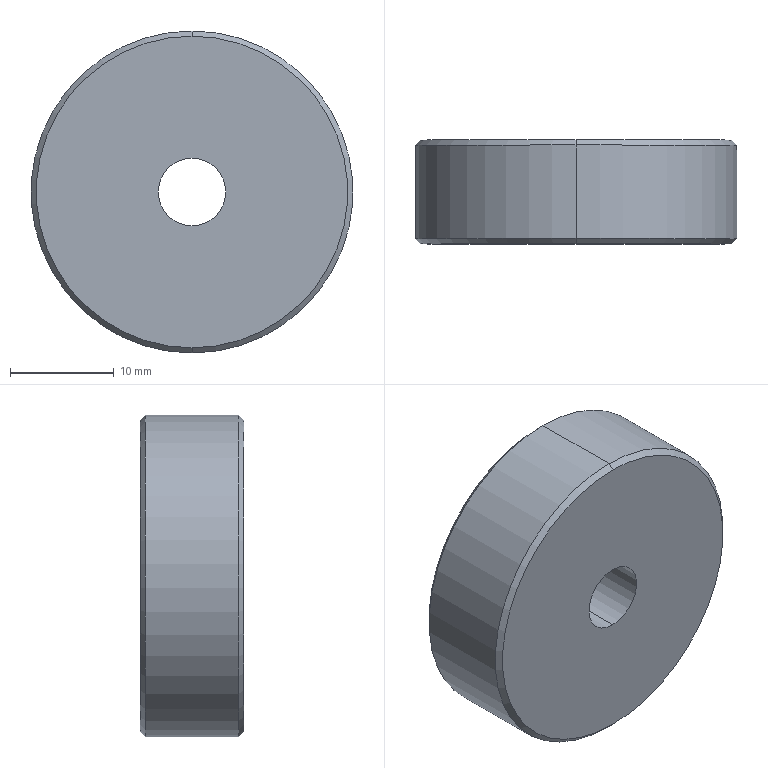Part | STEP file | OP10-124_seal pad | 1 solid | 13 faces | box 31 x 10 x 31 mm | volume 7003 mm3 | cylinder 6 | cone 4 | plane 3 | commonest cylinder face diameters 6.5 x2 9.5 x2 31 x2
STEP:
#1=CARTESIAN_POINT('',(0.,0.,0.));
#2=DIRECTION('',(0.,0.,1.));
#3=DIRECTION('',(1.,0.,0.));
#4=AXIS2_PLACEMENT_3D('',#1,#2,#3);
#5=CARTESIAN_POINT('',(0.,10.,15.));
#6=VERTEX_POINT('',#5);
#7=CARTESIAN_POINT('',(0.,10.,-15.));
#8=VERTEX_POINT('',#7);
#9=CARTESIAN_POINT('',(0.,10.,0.));
#10=DIRECTION('',(0.,1.,0.));
#11=DIRECTION('',(0.,0.,1.));
#12=AXIS2_PLACEMENT_3D('',#9,#10,#11);
#13=CIRCLE('',#12,15.);
#14=CARTESIAN_POINT('',(0.,10.,0.));
#15=DIRECTION('',(0.,-1.,0.));
#16=DIRECTION('',(0.,0.,-1.));
#17=AXIS2_PLACEMENT_3D('',#14,#15,#16);
#18=CONICAL_SURFACE('',#17,15.,0.7854);
#19=CARTESIAN_POINT('',(3.142,0.));
#20=DIRECTION('',(-1.,0.));
#21=VECTOR('',#20,1.);
#22=LINE('',#19,#21);
#23=(GEOMETRIC_REPRESENTATION_CONTEXT(2)PARAMETRIC_REPRESENTATION_CONTEXT()REPRESENTATION_CONTEXT('',''));
#24=DEFINITIONAL_REPRESENTATION('',(#22),#23);
#25=PCURVE('',#18,#24);
#26=CARTESIAN_POINT('',(0.,10.,0.));
#27=DIRECTION('',(0.,1.,0.));
#28=DIRECTION('',(0.,0.,1.));
#29=AXIS2_PLACEMENT_3D('',#26,#27,#28);
#30=PLANE('',#29);
#31=CARTESIAN_POINT('',(0.,0.));
#32=DIRECTION('',(1.,0.));
#33=AXIS2_PLACEMENT_2D('',#31,#32);
#34=CIRCLE('',#33,15.);
#35=(GEOMETRIC_REPRESENTATION_CONTEXT(2)PARAMETRIC_REPRESENTATION_CONTEXT()REPRESENTATION_CONTEXT('',''));
#36=DEFINITIONAL_REPRESENTATION('',(#34),#35);
#37=PCURVE('',#30,#36);
#38=SURFACE_CURVE('',#13,(#25,#37),.PCURVE_S1.);
#39=EDGE_CURVE('',#6,#8,#38,.T.);
#40=ORIENTED_EDGE('',*,*,#39,.F.);
#41=CARTESIAN_POINT('',(0.,9.5,15.5));
#42=VERTEX_POINT('',#41);
#43=CARTESIAN_POINT('',(0.,10.,15.));
#44=DIRECTION('',(0.,-0.7071,0.7071));
#45=VECTOR('',#44,1.);
#46=LINE('',#43,#45);
#47=CARTESIAN_POINT('',(3.142,0.));
#48=DIRECTION('',(0.,1.));
#49=VECTOR('',#48,1.);
#50=LINE('',#47,#49);
#51=(GEOMETRIC_REPRESENTATION_CONTEXT(2)PARAMETRIC_REPRESENTATION_CONTEXT()REPRESENTATION_CONTEXT('',''));
#52=DEFINITIONAL_REPRESENTATION('',(#50),#51);
#53=PCURVE('',#18,#52);
#54=CARTESIAN_POINT('',(0.,10.,0.));
#55=DIRECTION('',(0.,-1.,0.));
#56=DIRECTION('',(0.,0.,-1.));
#57=AXIS2_PLACEMENT_3D('',#54,#55,#56);
#58=CONICAL_SURFACE('',#57,15.,0.7854);
#59=CARTESIAN_POINT('',(3.142,0.));
#60=DIRECTION('',(0.,1.));
#61=VECTOR('',#60,1.);
#62=LINE('',#59,#61);
#63=(GEOMETRIC_REPRESENTATION_CONTEXT(2)PARAMETRIC_REPRESENTATION_CONTEXT()REPRESENTATION_CONTEXT('',''));
#64=DEFINITIONAL_REPRESENTATION('',(#62),#63);
#65=PCURVE('',#58,#64);
#66=SURFACE_CURVE('',#46,(#53,#65),.PCURVE_S1.);
#67=EDGE_CURVE('',#6,#42,#66,.T.);
#68=ORIENTED_EDGE('',*,*,#67,.T.);
#69=CARTESIAN_POINT('',(0.,9.5,-15.5));
#70=VERTEX_POINT('',#69);
#71=CARTESIAN_POINT('',(0.,9.5,0.));
#72=DIRECTION('',(0.,-1.,0.));
#73=DIRECTION('',(0.,0.,1.));
#74=AXIS2_PLACEMENT_3D('',#71,#72,#73);
#75=CIRCLE('',#74,15.5);
#76=CARTESIAN_POINT('',(-3.142,0.5));
#77=DIRECTION('',(1.,0.));
#78=VECTOR('',#77,1.);
#79=LINE('',#76,#78);
#80=(GEOMETRIC_REPRESENTATION_CONTEXT(2)PARAMETRIC_REPRESENTATION_CONTEXT()REPRESENTATION_CONTEXT('',''));
#81=DEFINITIONAL_REPRESENTATION('',(#79),#80);
#82=PCURVE('',#18,#81);
#83=CARTESIAN_POINT('',(0.,10.,0.));
#84=DIRECTION('',(0.,-1.,0.));
#85=DIRECTION('',(0.,0.,-1.));
#86=AXIS2_PLACEMENT_3D('',#83,#84,#85);
#87=CYLINDRICAL_SURFACE('',#86,15.5);
#88=CARTESIAN_POINT('',(-3.142,0.5));
#89=DIRECTION('',(1.,0.));
#90=VECTOR('',#89,1.);
#91=LINE('',#88,#90);
#92=(GEOMETRIC_REPRESENTATION_CONTEXT(2)PARAMETRIC_REPRESENTATION_CONTEXT()REPRESENTATION_CONTEXT('',''));
#93=DEFINITIONAL_REPRESENTATION('',(#91),#92);
#94=PCURVE('',#87,#93);
#95=SURFACE_CURVE('',#75,(#82,#94),.PCURVE_S1.);
#96=EDGE_CURVE('',#70,#42,#95,.T.);
#97=ORIENTED_EDGE('',*,*,#96,.F.);
#98=CARTESIAN_POINT('',(0.,10.,-15.));
#99=DIRECTION('',(0.,-0.7071,-0.7071));
#100=VECTOR('',#99,1.);
#101=LINE('',#98,#100);
#102=CARTESIAN_POINT('',(0.,0.));
#103=DIRECTION('',(0.,1.));
#104=VECTOR('',#103,1.);
#105=LINE('',#102,#104);
#106=(GEOMETRIC_REPRESENTATION_CONTEXT(2)PARAMETRIC_REPRESENTATION_CONTEXT()REPRESENTATION_CONTEXT('',''));
#107=DEFINITIONAL_REPRESENTATION('',(#105),#106);
#108=PCURVE('',#18,#107);
#109=CARTESIAN_POINT('',(6.283,0.));
#110=DIRECTION('',(0.,1.));
#111=VECTOR('',#110,1.);
#112=LINE('',#109,#111);
#113=(GEOMETRIC_REPRESENTATION_CONTEXT(2)PARAMETRIC_REPRESENTATION_CONTEXT()REPRESENTATION_CONTEXT('',''));
#114=DEFINITIONAL_REPRESENTATION('',(#112),#113);
#115=PCURVE('',#58,#114);
#116=SURFACE_CURVE('',#101,(#108,#115),.PCURVE_S1.);
#117=EDGE_CURVE('',#8,#70,#116,.T.);
#118=ORIENTED_EDGE('',*,*,#117,.F.);
#119=EDGE_LOOP('',(#40,#68,#97,#118));
#120=FACE_BOUND('',#119,.T.);
#121=ADVANCED_FACE('',(#120),#18,.T.);
#122=CARTESIAN_POINT('',(0.,0.,-15.));
#123=VERTEX_POINT('',#122);
#124=CARTESIAN_POINT('',(0.,0.,15.));
#125=VERTEX_POINT('',#124);
#126=CARTESIAN_POINT('',(0.,0.,0.));
#127=DIRECTION('',(0.,-1.,0.));
#128=DIRECTION('',(0.,0.,1.));
#129=AXIS2_PLACEMENT_3D('',#126,#127,#128);
#130=CIRCLE('',#129,15.);
#131=CARTESIAN_POINT('',(0.,0.5,0.));
#132=DIRECTION('',(0.,1.,0.));
#133=DIRECTION('',(0.,0.,1.));
#134=AXIS2_PLACEMENT_3D('',#131,#132,#133);
#135=CONICAL_SURFACE('',#134,15.5,0.7854);
#136=CARTESIAN_POINT('',(6.283,-0.5));
#137=DIRECTION('',(-1.,0.));
#138=VECTOR('',#137,1.);
#139=LINE('',#136,#138);
#140=(GEOMETRIC_REPRESENTATION_CONTEXT(2)PARAMETRIC_REPRESENTATION_CONTEXT()REPRESENTATION_CONTEXT('',''));
#141=DEFINITIONAL_REPRESENTATION('',(#139),#140);
#142=PCURVE('',#135,#141);
#143=CARTESIAN_POINT('',(0.,0.,0.));
#144=DIRECTION('',(0.,1.,0.));
#145=DIRECTION('',(0.,0.,1.));
#146=AXIS2_PLACEMENT_3D('',#143,#144,#145);
#147=PLANE('',#146);
#148=CARTESIAN_POINT('',(15.,0.));
#149=CARTESIAN_POINT('',(15.,-25.981));
#150=CARTESIAN_POINT('',(-7.5,-12.99));
#151=CARTESIAN_POINT('',(-30.,0.));
#152=CARTESIAN_POINT('',(-7.5,12.99));
#153=CARTESIAN_POINT('',(15.,25.981));
#154=CARTESIAN_POINT('',(15.,0.));
#155=(BOUNDED_CURVE()B_SPLINE_CURVE(2,(#148,#149,#150,#151,#152,#153,#154),.UNSPECIFIED.,.T.,.F.)B_SPLINE_CURVE_WITH_KNOTS((1,2,2,2,2,1),(-2.094,0.,2.094,4.189,6.283,8.378),.UNSPECIFIED.)CURVE()GEOMETRIC_REPRESENTATION_ITEM()RATIONAL_B_SPLINE_CURVE((1.,0.5,1.,0.5,1.,0.5,1.))REPRESENTATION_ITEM(''));
#156=(GEOMETRIC_REPRESENTATION_CONTEXT(2)PARAMETRIC_REPRESENTATION_CONTEXT()REPRESENTATION_CONTEXT('',''));
#157=DEFINITIONAL_REPRESENTATION('',(#155),#156);
#158=PCURVE('',#147,#157);
#159=SURFACE_CURVE('',#130,(#142,#158),.PCURVE_S1.);
#160=EDGE_CURVE('',#123,#125,#159,.T.);
#161=ORIENTED_EDGE('',*,*,#160,.F.);
#162=CARTESIAN_POINT('',(0.,0.5,-15.5));
#163=VERTEX_POINT('',#162);
#164=CARTESIAN_POINT('',(0.,0.5,-15.5));
#165=DIRECTION('',(0.,0.7071,-0.7071));
#166=VECTOR('',#165,1.);
#167=LINE('',#164,#166);
#168=CARTESIAN_POINT('',(3.142,0.));
#169=DIRECTION('',(0.,1.));
#170=VECTOR('',#169,1.);
#171=LINE('',#168,#170);
#172=(GEOMETRIC_REPRESENTATION_CONTEXT(2)PARAMETRIC_REPRESENTATION_CONTEXT()REPRESENTATION_CONTEXT('',''));
#173=DEFINITIONAL_REPRESENTATION('',(#171),#172);
#174=PCURVE('',#135,#173);
#175=CARTESIAN_POINT('',(0.,0.5,0.));
#176=DIRECTION('',(0.,1.,0.));
#177=DIRECTION('',(0.,0.,1.));
#178=AXIS2_PLACEMENT_3D('',#175,#176,#177);
#179=CONICAL_SURFACE('',#178,15.5,0.7854);
#180=CARTESIAN_POINT('',(3.142,0.));
#181=DIRECTION('',(0.,1.));
#182=VECTOR('',#181,1.);
#183=LINE('',#180,#182);
#184=(GEOMETRIC_REPRESENTATION_CONTEXT(2)PARAMETRIC_REPRESENTATION_CONTEXT()REPRESENTATION_CONTEXT('',''));
#185=DEFINITIONAL_REPRESENTATION('',(#183),#184);
#186=PCURVE('',#179,#185);
#187=SURFACE_CURVE('',#167,(#174,#186),.PCURVE_S1.);
#188=EDGE_CURVE('',#123,#163,#187,.T.);
#189=ORIENTED_EDGE('',*,*,#188,.T.);
#190=CARTESIAN_POINT('',(0.,0.5,15.5));
#191=VERTEX_POINT('',#190);
#192=CARTESIAN_POINT('',(0.,0.5,0.));
#193=DIRECTION('',(0.,1.,0.));
#194=DIRECTION('',(0.,0.,1.));
#195=AXIS2_PLACEMENT_3D('',#192,#193,#194);
#196=CIRCLE('',#195,15.5);
#197=CARTESIAN_POINT('',(0.,0.));
#198=DIRECTION('',(1.,0.));
#199=VECTOR('',#198,1.);
#200=LINE('',#197,#199);
#201=(GEOMETRIC_REPRESENTATION_CONTEXT(2)PARAMETRIC_REPRESENTATION_CONTEXT()REPRESENTATION_CONTEXT('',''));
#202=DEFINITIONAL_REPRESENTATION('',(#200),#201);
#203=PCURVE('',#135,#202);
#204=CARTESIAN_POINT('',(3.142,9.5));
#205=DIRECTION('',(-1.,0.));
#206=VECTOR('',#205,1.);
#207=LINE('',#204,#206);
#208=(GEOMETRIC_REPRESENTATION_CONTEXT(2)PARAMETRIC_REPRESENTATION_CONTEXT()REPRESENTATION_CONTEXT('',''));
#209=DEFINITIONAL_REPRESENTATION('',(#207),#208);
#210=PCURVE('',#87,#209);
#211=SURFACE_CURVE('',#196,(#203,#210),.PCURVE_S1.);
#212=EDGE_CURVE('',#191,#163,#211,.T.);
#213=ORIENTED_EDGE('',*,*,#212,.F.);
#214=CARTESIAN_POINT('',(0.,0.5,15.5));
#215=DIRECTION('',(0.,0.7071,0.7071));
#216=VECTOR('',#215,1.);
#217=LINE('',#214,#216);
#218=CARTESIAN_POINT('',(0.,0.));
#219=DIRECTION('',(0.,1.));
#220=VECTOR('',#219,1.);
#221=LINE('',#218,#220);
#222=(GEOMETRIC_REPRESENTATION_CONTEXT(2)PARAMETRIC_REPRESENTATION_CONTEXT()REPRESENTATION_CONTEXT('',''));
#223=DEFINITIONAL_REPRESENTATION('',(#221),#222);
#224=PCURVE('',#135,#223);
#225=CARTESIAN_POINT('',(6.283,0.));
#226=DIRECTION('',(0.,1.));
#227=VECTOR('',#226,1.);
#228=LINE('',#225,#227);
#229=(GEOMETRIC_REPRESENTATION_CONTEXT(2)PARAMETRIC_REPRESENTATION_CONTEXT()REPRESENTATION_CONTEXT('',''));
#230=DEFINITIONAL_REPRESENTATION('',(#228),#229);
#231=PCURVE('',#179,#230);
#232=SURFACE_CURVE('',#217,(#224,#231),.PCURVE_S1.);
#233=EDGE_CURVE('',#125,#191,#232,.T.);
#234=ORIENTED_EDGE('',*,*,#233,.F.);
#235=EDGE_LOOP('',(#161,#189,#213,#234));
#236=FACE_BOUND('',#235,.T.);
#237=ADVANCED_FACE('',(#236),#135,.T.);
#238=CARTESIAN_POINT('',(0.,5.,4.75));
#239=VERTEX_POINT('',#238);
#240=CARTESIAN_POINT('',(0.,10.,4.75));
#241=VERTEX_POINT('',#240);
#242=CARTESIAN_POINT('',(0.,5.,4.75));
#243=DIRECTION('',(0.,1.,0.));
#244=VECTOR('',#243,1.);
#245=LINE('',#242,#244);
#246=CARTESIAN_POINT('',(0.,5.,0.));
#247=DIRECTION('',(0.,1.,0.));
#248=DIRECTION('',(0.,0.,1.));
#249=AXIS2_PLACEMENT_3D('',#246,#247,#248);
#250=CYLINDRICAL_SURFACE('',#249,4.75);
#251=CARTESIAN_POINT('',(6.283,0.));
#252=DIRECTION('',(0.,1.));
#253=VECTOR('',#252,1.);
#254=LINE('',#251,#253);
#255=(GEOMETRIC_REPRESENTATION_CONTEXT(2)PARAMETRIC_REPRESENTATION_CONTEXT()REPRESENTATION_CONTEXT('',''));
#256=DEFINITIONAL_REPRESENTATION('',(#254),#255);
#257=PCURVE('',#250,#256);
#258=CARTESIAN_POINT('',(0.,5.,0.));
#259=DIRECTION('',(0.,1.,0.));
#260=DIRECTION('',(0.,0.,1.));
#261=AXIS2_PLACEMENT_3D('',#258,#259,#260);
#262=CYLINDRICAL_SURFACE('',#261,4.75);
#263=CARTESIAN_POINT('',(0.,0.));
#264=DIRECTION('',(0.,1.));
#265=VECTOR('',#264,1.);
#266=LINE('',#263,#265);
#267=(GEOMETRIC_REPRESENTATION_CONTEXT(2)PARAMETRIC_REPRESENTATION_CONTEXT()REPRESENTATION_CONTEXT('',''));
#268=DEFINITIONAL_REPRESENTATION('',(#266),#267);
#269=PCURVE('',#262,#268);
#270=SURFACE_CURVE('',#245,(#257,#269),.PCURVE_S1.);
#271=EDGE_CURVE('',#239,#241,#270,.T.);
#272=ORIENTED_EDGE('',*,*,#271,.T.);
#273=CARTESIAN_POINT('',(0.,10.,-4.75));
#274=VERTEX_POINT('',#273);
#275=CARTESIAN_POINT('',(0.,10.,0.));
#276=DIRECTION('',(0.,1.,0.));
#277=DIRECTION('',(0.,0.,1.));
#278=AXIS2_PLACEMENT_3D('',#275,#276,#277);
#279=CIRCLE('',#278,4.75);
#280=CARTESIAN_POINT('',(0.,5.));
#281=DIRECTION('',(1.,0.));
#282=VECTOR('',#281,1.);
#283=LINE('',#280,#282);
#284=(GEOMETRIC_REPRESENTATION_CONTEXT(2)PARAMETRIC_REPRESENTATION_CONTEXT()REPRESENTATION_CONTEXT('',''));
#285=DEFINITIONAL_REPRESENTATION('',(#283),#284);
#286=PCURVE('',#250,#285);
#287=CARTESIAN_POINT('',(0.,0.));
#288=DIRECTION('',(1.,0.));
#289=AXIS2_PLACEMENT_2D('',#287,#288);
#290=CIRCLE('',#289,4.75);
#291=(GEOMETRIC_REPRESENTATION_CONTEXT(2)PARAMETRIC_REPRESENTATION_CONTEXT()REPRESENTATION_CONTEXT('',''));
#292=DEFINITIONAL_REPRESENTATION('',(#290),#291);
#293=PCURVE('',#30,#292);
#294=SURFACE_CURVE('',#279,(#286,#293),.PCURVE_S1.);
#295=EDGE_CURVE('',#274,#241,#294,.T.);
#296=ORIENTED_EDGE('',*,*,#295,.F.);
#297=CARTESIAN_POINT('',(0.,5.,-4.75));
#298=VERTEX_POINT('',#297);
#299=CARTESIAN_POINT('',(0.,5.,-4.75));
#300=DIRECTION('',(0.,1.,0.));
#301=VECTOR('',#300,1.);
#302=LINE('',#299,#301);
#303=CARTESIAN_POINT('',(3.142,0.));
#304=DIRECTION('',(0.,1.));
#305=VECTOR('',#304,1.);
#306=LINE('',#303,#305);
#307=(GEOMETRIC_REPRESENTATION_CONTEXT(2)PARAMETRIC_REPRESENTATION_CONTEXT()REPRESENTATION_CONTEXT('',''));
#308=DEFINITIONAL_REPRESENTATION('',(#306),#307);
#309=PCURVE('',#250,#308);
#310=CARTESIAN_POINT('',(3.142,0.));
#311=DIRECTION('',(0.,1.));
#312=VECTOR('',#311,1.);
#313=LINE('',#310,#312);
#314=(GEOMETRIC_REPRESENTATION_CONTEXT(2)PARAMETRIC_REPRESENTATION_CONTEXT()REPRESENTATION_CONTEXT('',''));
#315=DEFINITIONAL_REPRESENTATION('',(#313),#314);
#316=PCURVE('',#262,#315);
#317=SURFACE_CURVE('',#302,(#309,#316),.PCURVE_S1.);
#318=EDGE_CURVE('',#298,#274,#317,.T.);
#319=ORIENTED_EDGE('',*,*,#318,.F.);
#320=CARTESIAN_POINT('',(0.,5.,0.));
#321=DIRECTION('',(0.,1.,0.));
#322=DIRECTION('',(0.,0.,1.));
#323=AXIS2_PLACEMENT_3D('',#320,#321,#322);
#324=CIRCLE('',#323,4.75);
#325=CARTESIAN_POINT('',(0.,0.));
#326=DIRECTION('',(1.,0.));
#327=VECTOR('',#326,1.);
#328=LINE('',#325,#327);
#329=(GEOMETRIC_REPRESENTATION_CONTEXT(2)PARAMETRIC_REPRESENTATION_CONTEXT()REPRESENTATION_CONTEXT('',''));
#330=DEFINITIONAL_REPRESENTATION('',(#328),#329);
#331=PCURVE('',#250,#330);
#332=CARTESIAN_POINT('',(0.,5.,0.));
#333=DIRECTION('',(0.,1.,0.));
#334=DIRECTION('',(0.,0.,1.));
#335=AXIS2_PLACEMENT_3D('',#332,#333,#334);
#336=PLANE('',#335);
#337=CARTESIAN_POINT('',(0.,0.));
#338=DIRECTION('',(1.,0.));
#339=AXIS2_PLACEMENT_2D('',#337,#338);
#340=CIRCLE('',#339,4.75);
#341=(GEOMETRIC_REPRESENTATION_CONTEXT(2)PARAMETRIC_REPRESENTATION_CONTEXT()REPRESENTATION_CONTEXT('',''));
#342=DEFINITIONAL_REPRESENTATION('',(#340),#341);
#343=PCURVE('',#336,#342);
#344=SURFACE_CURVE('',#324,(#331,#343),.PCURVE_S1.);
#345=EDGE_CURVE('',#298,#239,#344,.T.);
#346=ORIENTED_EDGE('',*,*,#345,.T.);
#347=EDGE_LOOP('',(#272,#296,#319,#346));
#348=FACE_BOUND('',#347,.F.);
#349=ADVANCED_FACE('',(#348),#250,.F.);
#350=ORIENTED_EDGE('',*,*,#96,.T.);
#351=CARTESIAN_POINT('',(0.,10.,15.5));
#352=DIRECTION('',(0.,-1.,0.));
#353=VECTOR('',#352,1.);
#354=LINE('',#351,#353);
#355=CARTESIAN_POINT('',(3.142,0.));
#356=DIRECTION('',(0.,1.));
#357=VECTOR('',#356,1.);
#358=LINE('',#355,#357);
#359=(GEOMETRIC_REPRESENTATION_CONTEXT(2)PARAMETRIC_REPRESENTATION_CONTEXT()REPRESENTATION_CONTEXT('',''));
#360=DEFINITIONAL_REPRESENTATION('',(#358),#359);
#361=PCURVE('',#87,#360);
#362=CARTESIAN_POINT('',(0.,10.,0.));
#363=DIRECTION('',(0.,-1.,0.));
#364=DIRECTION('',(0.,0.,-1.));
#365=AXIS2_PLACEMENT_3D('',#362,#363,#364);
#366=CYLINDRICAL_SURFACE('',#365,15.5);
#367=CARTESIAN_POINT('',(3.142,0.));
#368=DIRECTION('',(0.,1.));
#369=VECTOR('',#368,1.);
#370=LINE('',#367,#369);
#371=(GEOMETRIC_REPRESENTATION_CONTEXT(2)PARAMETRIC_REPRESENTATION_CONTEXT()REPRESENTATION_CONTEXT('',''));
#372=DEFINITIONAL_REPRESENTATION('',(#370),#371);
#373=PCURVE('',#366,#372);
#374=SURFACE_CURVE('',#354,(#361,#373),.PCURVE_S1.);
#375=EDGE_CURVE('',#42,#191,#374,.T.);
#376=ORIENTED_EDGE('',*,*,#375,.T.);
#377=ORIENTED_EDGE('',*,*,#212,.T.);
#378=CARTESIAN_POINT('',(0.,10.,-15.5));
#379=DIRECTION('',(0.,-1.,0.));
#380=VECTOR('',#379,1.);
#381=LINE('',#378,#380);
#382=CARTESIAN_POINT('',(0.,0.));
#383=DIRECTION('',(0.,1.));
#384=VECTOR('',#383,1.);
#385=LINE('',#382,#384);
#386=(GEOMETRIC_REPRESENTATION_CONTEXT(2)PARAMETRIC_REPRESENTATION_CONTEXT()REPRESENTATION_CONTEXT('',''));
#387=DEFINITIONAL_REPRESENTATION('',(#385),#386);
#388=PCURVE('',#87,#387);
#389=CARTESIAN_POINT('',(6.283,0.));
#390=DIRECTION('',(0.,1.));
#391=VECTOR('',#390,1.);
#392=LINE('',#389,#391);
#393=(GEOMETRIC_REPRESENTATION_CONTEXT(2)PARAMETRIC_REPRESENTATION_CONTEXT()REPRESENTATION_CONTEXT('',''));
#394=DEFINITIONAL_REPRESENTATION('',(#392),#393);
#395=PCURVE('',#366,#394);
#396=SURFACE_CURVE('',#381,(#388,#395),.PCURVE_S1.);
#397=EDGE_CURVE('',#70,#163,#396,.T.);
#398=ORIENTED_EDGE('',*,*,#397,.F.);
#399=EDGE_LOOP('',(#350,#376,#377,#398));
#400=FACE_BOUND('',#399,.T.);
#401=ADVANCED_FACE('',(#400),#87,.T.);
#402=CARTESIAN_POINT('',(0.,5.,-3.25));
#403=VERTEX_POINT('',#402);
#404=CARTESIAN_POINT('',(0.,0.,-3.25));
#405=VERTEX_POINT('',#404);
#406=CARTESIAN_POINT('',(0.,10.,-3.25));
#407=DIRECTION('',(0.,-1.,0.));
#408=VECTOR('',#407,1.);
#409=LINE('',#406,#408);
#410=CARTESIAN_POINT('',(0.,10.,0.));
#411=DIRECTION('',(0.,-1.,0.));
#412=DIRECTION('',(0.,0.,-1.));
#413=AXIS2_PLACEMENT_3D('',#410,#411,#412);
#414=CYLINDRICAL_SURFACE('',#413,3.25);
#415=CARTESIAN_POINT('',(6.283,0.));
#416=DIRECTION('',(0.,1.));
#417=VECTOR('',#416,1.);
#418=LINE('',#415,#417);
#419=(GEOMETRIC_REPRESENTATION_CONTEXT(2)PARAMETRIC_REPRESENTATION_CONTEXT()REPRESENTATION_CONTEXT('',''));
#420=DEFINITIONAL_REPRESENTATION('',(#418),#419);
#421=PCURVE('',#414,#420);
#422=CARTESIAN_POINT('',(0.,10.,0.));
#423=DIRECTION('',(0.,-1.,0.));
#424=DIRECTION('',(0.,0.,-1.));
#425=AXIS2_PLACEMENT_3D('',#422,#423,#424);
#426=CYLINDRICAL_SURFACE('',#425,3.25);
#427=CARTESIAN_POINT('',(0.,0.));
#428=DIRECTION('',(0.,1.));
#429=VECTOR('',#428,1.);
#430=LINE('',#427,#429);
#431=(GEOMETRIC_REPRESENTATION_CONTEXT(2)PARAMETRIC_REPRESENTATION_CONTEXT()REPRESENTATION_CONTEXT('',''));
#432=DEFINITIONAL_REPRESENTATION('',(#430),#431);
#433=PCURVE('',#426,#432);
#434=SURFACE_CURVE('',#409,(#421,#433),.PCURVE_S1.);
#435=EDGE_CURVE('',#403,#405,#434,.T.);
#436=ORIENTED_EDGE('',*,*,#435,.T.);
#437=CARTESIAN_POINT('',(0.,0.,3.25));
#438=VERTEX_POINT('',#437);
#439=CARTESIAN_POINT('',(0.,0.,0.));
#440=DIRECTION('',(0.,1.,0.));
#441=DIRECTION('',(0.,0.,1.));
#442=AXIS2_PLACEMENT_3D('',#439,#440,#441);
#443=CIRCLE('',#442,3.25);
#444=CARTESIAN_POINT('',(9.425,10.));
#445=DIRECTION('',(-1.,0.));
#446=VECTOR('',#445,1.);
#447=LINE('',#444,#446);
#448=(GEOMETRIC_REPRESENTATION_CONTEXT(2)PARAMETRIC_REPRESENTATION_CONTEXT()REPRESENTATION_CONTEXT('',''));
#449=DEFINITIONAL_REPRESENTATION('',(#447),#448);
#450=PCURVE('',#414,#449);
#451=CARTESIAN_POINT('',(0.,0.));
#452=DIRECTION('',(1.,0.));
#453=AXIS2_PLACEMENT_2D('',#451,#452);
#454=CIRCLE('',#453,3.25);
#455=(GEOMETRIC_REPRESENTATION_CONTEXT(2)PARAMETRIC_REPRESENTATION_CONTEXT()REPRESENTATION_CONTEXT('',''));
#456=DEFINITIONAL_REPRESENTATION('',(#454),#455);
#457=PCURVE('',#147,#456);
#458=SURFACE_CURVE('',#443,(#450,#457),.PCURVE_S1.);
#459=EDGE_CURVE('',#405,#438,#458,.T.);
#460=ORIENTED_EDGE('',*,*,#459,.T.);
#461=CARTESIAN_POINT('',(0.,5.,3.25));
#462=VERTEX_POINT('',#461);
#463=CARTESIAN_POINT('',(0.,10.,3.25));
#464=DIRECTION('',(0.,-1.,0.));
#465=VECTOR('',#464,1.);
#466=LINE('',#463,#465);
#467=CARTESIAN_POINT('',(3.142,0.));
#468=DIRECTION('',(0.,1.));
#469=VECTOR('',#468,1.);
#470=LINE('',#467,#469);
#471=(GEOMETRIC_REPRESENTATION_CONTEXT(2)PARAMETRIC_REPRESENTATION_CONTEXT()REPRESENTATION_CONTEXT('',''));
#472=DEFINITIONAL_REPRESENTATION('',(#470),#471);
#473=PCURVE('',#414,#472);
#474=CARTESIAN_POINT('',(3.142,0.));
#475=DIRECTION('',(0.,1.));
#476=VECTOR('',#475,1.);
#477=LINE('',#474,#476);
#478=(GEOMETRIC_REPRESENTATION_CONTEXT(2)PARAMETRIC_REPRESENTATION_CONTEXT()REPRESENTATION_CONTEXT('',''));
#479=DEFINITIONAL_REPRESENTATION('',(#477),#478);
#480=PCURVE('',#426,#479);
#481=SURFACE_CURVE('',#466,(#473,#480),.PCURVE_S1.);
#482=EDGE_CURVE('',#462,#438,#481,.T.);
#483=ORIENTED_EDGE('',*,*,#482,.F.);
#484=CARTESIAN_POINT('',(0.,5.,0.));
#485=DIRECTION('',(0.,1.,0.));
#486=DIRECTION('',(0.,0.,1.));
#487=AXIS2_PLACEMENT_3D('',#484,#485,#486);
#488=CIRCLE('',#487,3.25);
#489=CARTESIAN_POINT('',(9.425,5.));
#490=DIRECTION('',(-1.,0.));
#491=VECTOR('',#490,1.);
#492=LINE('',#489,#491);
#493=(GEOMETRIC_REPRESENTATION_CONTEXT(2)PARAMETRIC_REPRESENTATION_CONTEXT()REPRESENTATION_CONTEXT('',''));
#494=DEFINITIONAL_REPRESENTATION('',(#492),#493);
#495=PCURVE('',#414,#494);
#496=CARTESIAN_POINT('',(0.,0.));
#497=DIRECTION('',(1.,0.));
#498=AXIS2_PLACEMENT_2D('',#496,#497);
#499=CIRCLE('',#498,3.25);
#500=(GEOMETRIC_REPRESENTATION_CONTEXT(2)PARAMETRIC_REPRESENTATION_CONTEXT()REPRESENTATION_CONTEXT('',''));
#501=DEFINITIONAL_REPRESENTATION('',(#499),#500);
#502=PCURVE('',#336,#501);
#503=SURFACE_CURVE('',#488,(#495,#502),.PCURVE_S1.);
#504=EDGE_CURVE('',#403,#462,#503,.T.);
#505=ORIENTED_EDGE('',*,*,#504,.F.);
#506=EDGE_LOOP('',(#436,#460,#483,#505));
#507=FACE_BOUND('',#506,.F.);
#508=ADVANCED_FACE('',(#507),#414,.F.);
#509=CARTESIAN_POINT('',(0.,0.,0.));
#510=DIRECTION('',(0.,1.,0.));
#511=DIRECTION('',(0.,0.,1.));
#512=AXIS2_PLACEMENT_3D('',#509,#510,#511);
#513=CIRCLE('',#512,3.25);
#514=CARTESIAN_POINT('',(3.142,10.));
#515=DIRECTION('',(-1.,0.));
#516=VECTOR('',#515,1.);
#517=LINE('',#514,#516);
#518=(GEOMETRIC_REPRESENTATION_CONTEXT(2)PARAMETRIC_REPRESENTATION_CONTEXT()REPRESENTATION_CONTEXT('',''));
#519=DEFINITIONAL_REPRESENTATION('',(#517),#518);
#520=PCURVE('',#426,#519);
#521=CARTESIAN_POINT('',(0.,0.));
#522=DIRECTION('',(1.,0.));
#523=AXIS2_PLACEMENT_2D('',#521,#522);
#524=CIRCLE('',#523,3.25);
#525=(GEOMETRIC_REPRESENTATION_CONTEXT(2)PARAMETRIC_REPRESENTATION_CONTEXT()REPRESENTATION_CONTEXT('',''));
#526=DEFINITIONAL_REPRESENTATION('',(#524),#525);
#527=PCURVE('',#147,#526);
#528=SURFACE_CURVE('',#513,(#520,#527),.PCURVE_S1.);
#529=EDGE_CURVE('',#438,#405,#528,.T.);
#530=ORIENTED_EDGE('',*,*,#529,.T.);
#531=ORIENTED_EDGE('',*,*,#435,.F.);
#532=CARTESIAN_POINT('',(0.,5.,0.));
#533=DIRECTION('',(0.,1.,0.));
#534=DIRECTION('',(0.,0.,1.));
#535=AXIS2_PLACEMENT_3D('',#532,#533,#534);
#536=CIRCLE('',#535,3.25);
#537=CARTESIAN_POINT('',(3.142,5.));
#538=DIRECTION('',(-1.,0.));
#539=VECTOR('',#538,1.);
#540=LINE('',#537,#539);
#541=(GEOMETRIC_REPRESENTATION_CONTEXT(2)PARAMETRIC_REPRESENTATION_CONTEXT()REPRESENTATION_CONTEXT('',''));
#542=DEFINITIONAL_REPRESENTATION('',(#540),#541);
#543=PCURVE('',#426,#542);
#544=CARTESIAN_POINT('',(0.,0.));
#545=DIRECTION('',(1.,0.));
#546=AXIS2_PLACEMENT_2D('',#544,#545);
#547=CIRCLE('',#546,3.25);
#548=(GEOMETRIC_REPRESENTATION_CONTEXT(2)PARAMETRIC_REPRESENTATION_CONTEXT()REPRESENTATION_CONTEXT('',''));
#549=DEFINITIONAL_REPRESENTATION('',(#547),#548);
#550=PCURVE('',#336,#549);
#551=SURFACE_CURVE('',#536,(#543,#550),.PCURVE_S1.);
#552=EDGE_CURVE('',#462,#403,#551,.T.);
#553=ORIENTED_EDGE('',*,*,#552,.F.);
#554=ORIENTED_EDGE('',*,*,#482,.T.);
#555=EDGE_LOOP('',(#530,#531,#553,#554));
#556=FACE_BOUND('',#555,.F.);
#557=ADVANCED_FACE('',(#556),#426,.F.);
#558=CARTESIAN_POINT('',(0.,10.,0.));
#559=DIRECTION('',(0.,1.,0.));
#560=DIRECTION('',(0.,0.,1.));
#561=AXIS2_PLACEMENT_3D('',#558,#559,#560);
#562=CIRCLE('',#561,15.);
#563=CARTESIAN_POINT('',(0.,0.));
#564=DIRECTION('',(1.,0.));
#565=AXIS2_PLACEMENT_2D('',#563,#564);
#566=CIRCLE('',#565,15.);
#567=(GEOMETRIC_REPRESENTATION_CONTEXT(2)PARAMETRIC_REPRESENTATION_CONTEXT()REPRESENTATION_CONTEXT('',''));
#568=DEFINITIONAL_REPRESENTATION('',(#566),#567);
#569=PCURVE('',#30,#568);
#570=CARTESIAN_POINT('',(9.425,0.));
#571=DIRECTION('',(-1.,0.));
#572=VECTOR('',#571,1.);
#573=LINE('',#570,#572);
#574=(GEOMETRIC_REPRESENTATION_CONTEXT(2)PARAMETRIC_REPRESENTATION_CONTEXT()REPRESENTATION_CONTEXT('',''));
#575=DEFINITIONAL_REPRESENTATION('',(#573),#574);
#576=PCURVE('',#58,#575);
#577=SURFACE_CURVE('',#562,(#569,#576),.PCURVE_S1.);
#578=EDGE_CURVE('',#8,#6,#577,.T.);
#579=ORIENTED_EDGE('',*,*,#578,.T.);
#580=ORIENTED_EDGE('',*,*,#39,.T.);
#581=EDGE_LOOP('',(#579,#580));
#582=FACE_BOUND('',#581,.T.);
#583=CARTESIAN_POINT('',(0.,10.,0.));
#584=DIRECTION('',(0.,1.,0.));
#585=DIRECTION('',(0.,0.,1.));
#586=AXIS2_PLACEMENT_3D('',#583,#584,#585);
#587=CIRCLE('',#586,4.75);
#588=CARTESIAN_POINT('',(0.,0.));
#589=DIRECTION('',(1.,0.));
#590=AXIS2_PLACEMENT_2D('',#588,#589);
#591=CIRCLE('',#590,4.75);
#592=(GEOMETRIC_REPRESENTATION_CONTEXT(2)PARAMETRIC_REPRESENTATION_CONTEXT()REPRESENTATION_CONTEXT('',''));
#593=DEFINITIONAL_REPRESENTATION('',(#591),#592);
#594=PCURVE('',#30,#593);
#595=CARTESIAN_POINT('',(0.,5.));
#596=DIRECTION('',(1.,0.));
#597=VECTOR('',#596,1.);
#598=LINE('',#595,#597);
#599=(GEOMETRIC_REPRESENTATION_CONTEXT(2)PARAMETRIC_REPRESENTATION_CONTEXT()REPRESENTATION_CONTEXT('',''));
#600=DEFINITIONAL_REPRESENTATION('',(#598),#599);
#601=PCURVE('',#262,#600);
#602=SURFACE_CURVE('',#587,(#594,#601),.PCURVE_S1.);
#603=EDGE_CURVE('',#241,#274,#602,.T.);
#604=ORIENTED_EDGE('',*,*,#603,.F.);
#605=ORIENTED_EDGE('',*,*,#295,.F.);
#606=EDGE_LOOP('',(#604,#605));
#607=FACE_BOUND('',#606,.T.);
#608=ADVANCED_FACE('',(#582,#607),#30,.T.);
#609=CARTESIAN_POINT('',(0.,0.,0.));
#610=DIRECTION('',(0.,-1.,0.));
#611=DIRECTION('',(0.,0.,1.));
#612=AXIS2_PLACEMENT_3D('',#609,#610,#611);
#613=CIRCLE('',#612,15.);
#614=CARTESIAN_POINT('',(15.,0.));
#615=CARTESIAN_POINT('',(15.,-25.981));
#616=CARTESIAN_POINT('',(-7.5,-12.99));
#617=CARTESIAN_POINT('',(-30.,0.));
#618=CARTESIAN_POINT('',(-7.5,12.99));
#619=CARTESIAN_POINT('',(15.,25.981));
#620=CARTESIAN_POINT('',(15.,0.));
#621=(BOUNDED_CURVE()B_SPLINE_CURVE(2,(#614,#615,#616,#617,#618,#619,#620),.UNSPECIFIED.,.T.,.F.)B_SPLINE_CURVE_WITH_KNOTS((1,2,2,2,2,1),(-2.094,0.,2.094,4.189,6.283,8.378),.UNSPECIFIED.)CURVE()GEOMETRIC_REPRESENTATION_ITEM()RATIONAL_B_SPLINE_CURVE((1.,0.5,1.,0.5,1.,0.5,1.))REPRESENTATION_ITEM(''));
#622=(GEOMETRIC_REPRESENTATION_CONTEXT(2)PARAMETRIC_REPRESENTATION_CONTEXT()REPRESENTATION_CONTEXT('',''));
#623=DEFINITIONAL_REPRESENTATION('',(#621),#622);
#624=PCURVE('',#147,#623);
#625=CARTESIAN_POINT('',(6.283,-0.5));
#626=DIRECTION('',(-1.,0.));
#627=VECTOR('',#626,1.);
#628=LINE('',#625,#627);
#629=(GEOMETRIC_REPRESENTATION_CONTEXT(2)PARAMETRIC_REPRESENTATION_CONTEXT()REPRESENTATION_CONTEXT('',''));
#630=DEFINITIONAL_REPRESENTATION('',(#628),#629);
#631=PCURVE('',#179,#630);
#632=SURFACE_CURVE('',#613,(#624,#631),.PCURVE_S1.);
#633=EDGE_CURVE('',#125,#123,#632,.T.);
#634=ORIENTED_EDGE('',*,*,#633,.T.);
#635=ORIENTED_EDGE('',*,*,#160,.T.);
#636=EDGE_LOOP('',(#634,#635));
#637=FACE_BOUND('',#636,.T.);
#638=ORIENTED_EDGE('',*,*,#459,.T.);
#639=ORIENTED_EDGE('',*,*,#529,.T.);
#640=EDGE_LOOP('',(#638,#639));
#641=FACE_BOUND('',#640,.T.);
#642=ADVANCED_FACE('',(#637,#641),#147,.F.);
#643=ORIENTED_EDGE('',*,*,#375,.F.);
#644=CARTESIAN_POINT('',(0.,9.5,0.));
#645=DIRECTION('',(0.,-1.,0.));
#646=DIRECTION('',(0.,0.,1.));
#647=AXIS2_PLACEMENT_3D('',#644,#645,#646);
#648=CIRCLE('',#647,15.5);
#649=CARTESIAN_POINT('',(3.142,0.5));
#650=DIRECTION('',(1.,0.));
#651=VECTOR('',#650,1.);
#652=LINE('',#649,#651);
#653=(GEOMETRIC_REPRESENTATION_CONTEXT(2)PARAMETRIC_REPRESENTATION_CONTEXT()REPRESENTATION_CONTEXT('',''));
#654=DEFINITIONAL_REPRESENTATION('',(#652),#653);
#655=PCURVE('',#366,#654);
#656=CARTESIAN_POINT('',(3.142,0.5));
#657=DIRECTION('',(1.,0.));
#658=VECTOR('',#657,1.);
#659=LINE('',#656,#658);
#660=(GEOMETRIC_REPRESENTATION_CONTEXT(2)PARAMETRIC_REPRESENTATION_CONTEXT()REPRESENTATION_CONTEXT('',''));
#661=DEFINITIONAL_REPRESENTATION('',(#659),#660);
#662=PCURVE('',#58,#661);
#663=SURFACE_CURVE('',#648,(#655,#662),.PCURVE_S1.);
#664=EDGE_CURVE('',#42,#70,#663,.T.);
#665=ORIENTED_EDGE('',*,*,#664,.T.);
#666=ORIENTED_EDGE('',*,*,#397,.T.);
#667=CARTESIAN_POINT('',(0.,0.5,0.));
#668=DIRECTION('',(0.,1.,0.));
#669=DIRECTION('',(0.,0.,1.));
#670=AXIS2_PLACEMENT_3D('',#667,#668,#669);
#671=CIRCLE('',#670,15.5);
#672=CARTESIAN_POINT('',(9.425,9.5));
#673=DIRECTION('',(-1.,0.));
#674=VECTOR('',#673,1.);
#675=LINE('',#672,#674);
#676=(GEOMETRIC_REPRESENTATION_CONTEXT(2)PARAMETRIC_REPRESENTATION_CONTEXT()REPRESENTATION_CONTEXT('',''));
#677=DEFINITIONAL_REPRESENTATION('',(#675),#676);
#678=PCURVE('',#366,#677);
#679=CARTESIAN_POINT('',(0.,0.));
#680=DIRECTION('',(1.,0.));
#681=VECTOR('',#680,1.);
#682=LINE('',#679,#681);
#683=(GEOMETRIC_REPRESENTATION_CONTEXT(2)PARAMETRIC_REPRESENTATION_CONTEXT()REPRESENTATION_CONTEXT('',''));
#684=DEFINITIONAL_REPRESENTATION('',(#682),#683);
#685=PCURVE('',#179,#684);
#686=SURFACE_CURVE('',#671,(#678,#685),.PCURVE_S1.);
#687=EDGE_CURVE('',#163,#191,#686,.T.);
#688=ORIENTED_EDGE('',*,*,#687,.T.);
#689=EDGE_LOOP('',(#643,#665,#666,#688));
#690=FACE_BOUND('',#689,.T.);
#691=ADVANCED_FACE('',(#690),#366,.T.);
#692=ORIENTED_EDGE('',*,*,#603,.F.);
#693=ORIENTED_EDGE('',*,*,#271,.F.);
#694=CARTESIAN_POINT('',(0.,5.,0.));
#695=DIRECTION('',(0.,1.,0.));
#696=DIRECTION('',(0.,0.,1.));
#697=AXIS2_PLACEMENT_3D('',#694,#695,#696);
#698=CIRCLE('',#697,4.75);
#699=CARTESIAN_POINT('',(0.,0.));
#700=DIRECTION('',(1.,0.));
#701=VECTOR('',#700,1.);
#702=LINE('',#699,#701);
#703=(GEOMETRIC_REPRESENTATION_CONTEXT(2)PARAMETRIC_REPRESENTATION_CONTEXT()REPRESENTATION_CONTEXT('',''));
#704=DEFINITIONAL_REPRESENTATION('',(#702),#703);
#705=PCURVE('',#262,#704);
#706=CARTESIAN_POINT('',(0.,0.));
#707=DIRECTION('',(1.,0.));
#708=AXIS2_PLACEMENT_2D('',#706,#707);
#709=CIRCLE('',#708,4.75);
#710=(GEOMETRIC_REPRESENTATION_CONTEXT(2)PARAMETRIC_REPRESENTATION_CONTEXT()REPRESENTATION_CONTEXT('',''));
#711=DEFINITIONAL_REPRESENTATION('',(#709),#710);
#712=PCURVE('',#336,#711);
#713=SURFACE_CURVE('',#698,(#705,#712),.PCURVE_S1.);
#714=EDGE_CURVE('',#239,#298,#713,.T.);
#715=ORIENTED_EDGE('',*,*,#714,.T.);
#716=ORIENTED_EDGE('',*,*,#318,.T.);
#717=EDGE_LOOP('',(#692,#693,#715,#716));
#718=FACE_BOUND('',#717,.F.);
#719=ADVANCED_FACE('',(#718),#262,.F.);
#720=ORIENTED_EDGE('',*,*,#504,.F.);
#721=ORIENTED_EDGE('',*,*,#552,.F.);
#722=EDGE_LOOP('',(#720,#721));
#723=FACE_BOUND('',#722,.T.);
#724=ORIENTED_EDGE('',*,*,#714,.T.);
#725=ORIENTED_EDGE('',*,*,#345,.T.);
#726=EDGE_LOOP('',(#724,#725));
#727=FACE_BOUND('',#726,.T.);
#728=ADVANCED_FACE('',(#723,#727),#336,.T.);
#729=ORIENTED_EDGE('',*,*,#188,.F.);
#730=ORIENTED_EDGE('',*,*,#633,.F.);
#731=ORIENTED_EDGE('',*,*,#233,.T.);
#732=ORIENTED_EDGE('',*,*,#687,.F.);
#733=EDGE_LOOP('',(#729,#730,#731,#732));
#734=FACE_BOUND('',#733,.T.);
#735=ADVANCED_FACE('',(#734),#179,.T.);
#736=ORIENTED_EDGE('',*,*,#67,.F.);
#737=ORIENTED_EDGE('',*,*,#578,.F.);
#738=ORIENTED_EDGE('',*,*,#117,.T.);
#739=ORIENTED_EDGE('',*,*,#664,.F.);
#740=EDGE_LOOP('',(#736,#737,#738,#739));
#741=FACE_BOUND('',#740,.T.);
#742=ADVANCED_FACE('',(#741),#58,.T.);
#743=CLOSED_SHELL('',(#121,#237,#349,#401,#508,#557,#608,#642,#691,#719,#728,#735,#742));
#744=MANIFOLD_SOLID_BREP('',#743);
#745=(LENGTH_UNIT()NAMED_UNIT(*)SI_UNIT(.MILLI.,.METRE.));
#746=UNCERTAINTY_MEASURE_WITH_UNIT(LENGTH_MEASURE(0.0000001),#745,'','');
#747=(NAMED_UNIT(*)PLANE_ANGLE_UNIT()SI_UNIT($,.RADIAN.));
#748=(NAMED_UNIT(*)SI_UNIT($,.STERADIAN.)SOLID_ANGLE_UNIT());
#749=(GEOMETRIC_REPRESENTATION_CONTEXT(3)GLOBAL_UNCERTAINTY_ASSIGNED_CONTEXT((#746))GLOBAL_UNIT_ASSIGNED_CONTEXT((#745,#747,#748))REPRESENTATION_CONTEXT('',''));
#750=ADVANCED_BREP_SHAPE_REPRESENTATION('',(#4,#744),#749);